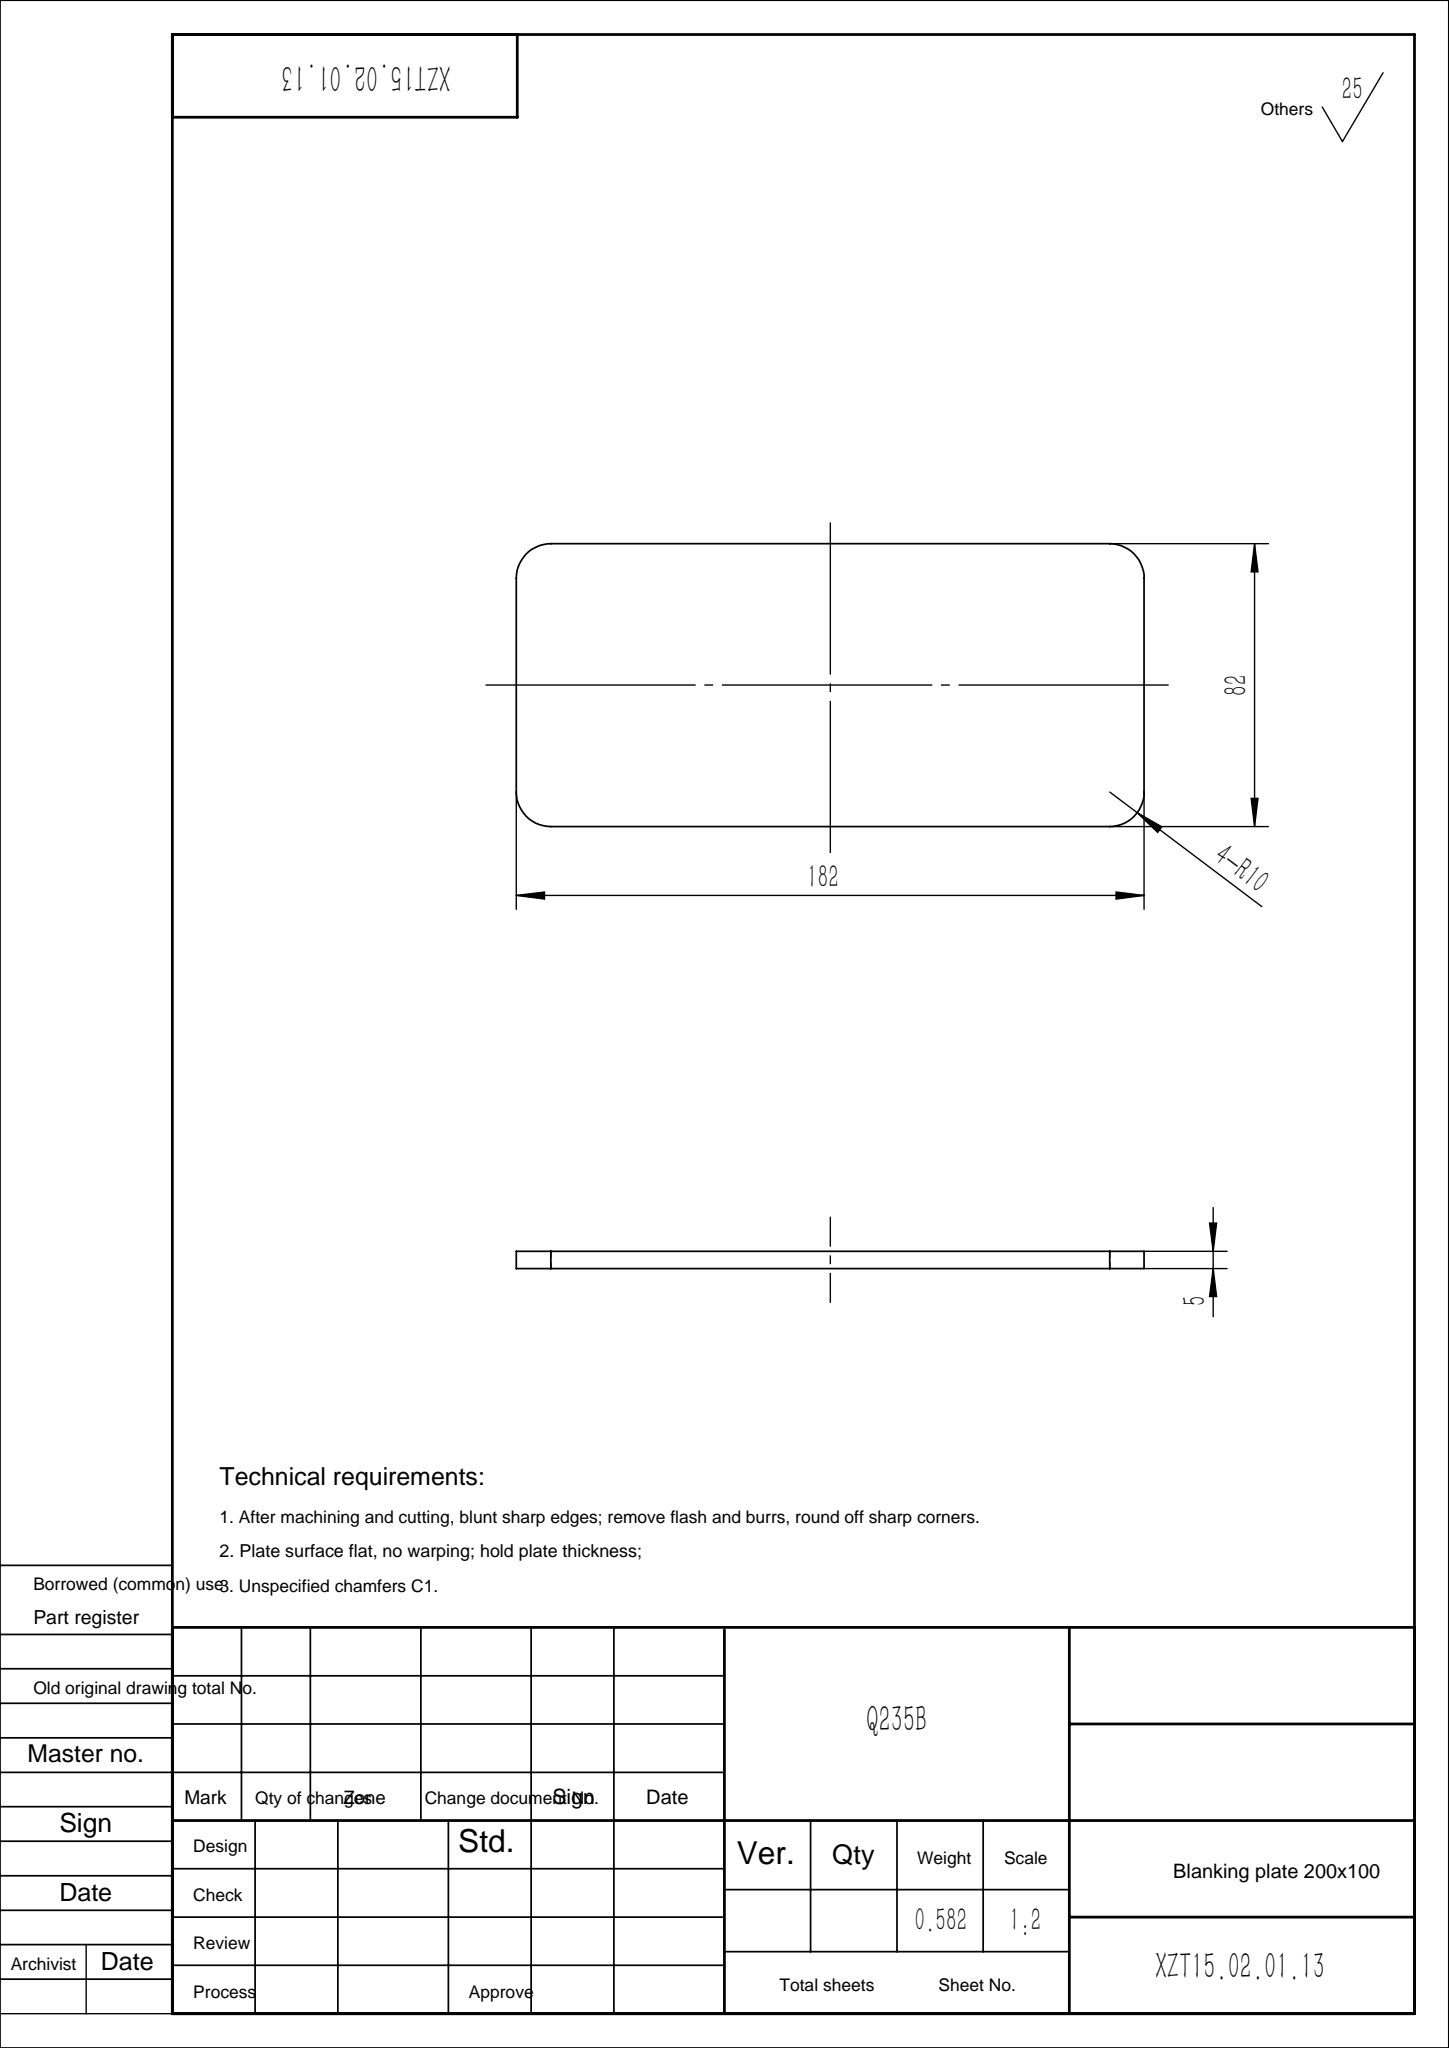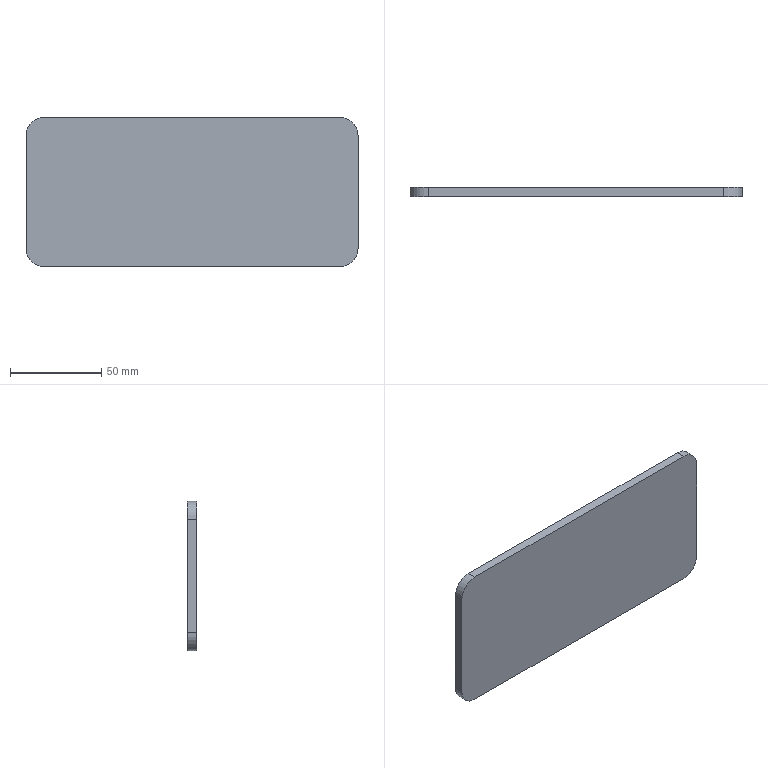Part | SolidWorks | features Chamfer 1, Extrusion 1, Fillet 1, HoleWzd 1 | 1 solid | 10 faces | box 182 x 5 x 82 mm | volume 74191 mm3 | plane 6 | cylinder 4 | commonest cylinder face diameters 20 x4
STEP:
#1=CARTESIAN_POINT('',(-91.,0.,-31.));
#2=VERTEX_POINT('',#1);
#3=CARTESIAN_POINT('',(-91.,0.,31.));
#4=VERTEX_POINT('',#3);
#5=CARTESIAN_POINT('',(-91.,0.,41.));
#6=DIRECTION('',(0.,0.,1.));
#7=VECTOR('',#6,1000.);
#8=LINE('',#5,#7);
#9=EDGE_CURVE('',#2,#4,#8,.T.);
#10=ORIENTED_EDGE('',*,*,#9,.T.);
#11=CARTESIAN_POINT('',(-91.,5.,31.));
#12=VERTEX_POINT('',#11);
#13=CARTESIAN_POINT('',(-91.,5.,31.));
#14=DIRECTION('',(0.,1.,0.));
#15=VECTOR('',#14,1000.);
#16=LINE('',#13,#15);
#17=EDGE_CURVE('',#4,#12,#16,.T.);
#18=ORIENTED_EDGE('',*,*,#17,.T.);
#19=CARTESIAN_POINT('',(-91.,5.,-31.));
#20=VERTEX_POINT('',#19);
#21=CARTESIAN_POINT('',(-91.,5.,41.));
#22=DIRECTION('',(0.,0.,1.));
#23=VECTOR('',#22,1000.);
#24=LINE('',#21,#23);
#25=EDGE_CURVE('',#20,#12,#24,.T.);
#26=ORIENTED_EDGE('',*,*,#25,.F.);
#27=CARTESIAN_POINT('',(-91.,5.,-31.));
#28=DIRECTION('',(0.,-1.,0.));
#29=VECTOR('',#28,1000.);
#30=LINE('',#27,#29);
#31=EDGE_CURVE('',#20,#2,#30,.T.);
#32=ORIENTED_EDGE('',*,*,#31,.T.);
#33=EDGE_LOOP('',(#10,#18,#26,#32));
#34=FACE_OUTER_BOUND('',#33,.T.);
#35=CARTESIAN_POINT('',(-91.,5.,41.));
#36=DIRECTION('',(1.,0.,0.));
#37=DIRECTION('',(0.,0.,-1.));
#38=AXIS2_PLACEMENT_3D('',#35,#36,#37);
#39=PLANE('',#38);
#40=ADVANCED_FACE('',(#34),#39,.F.);
#41=CARTESIAN_POINT('',(-81.,0.,41.));
#42=VERTEX_POINT('',#41);
#43=CARTESIAN_POINT('',(81.,0.,41.));
#44=VERTEX_POINT('',#43);
#45=CARTESIAN_POINT('',(91.,0.,41.));
#46=DIRECTION('',(1.,0.,0.));
#47=VECTOR('',#46,1000.);
#48=LINE('',#45,#47);
#49=EDGE_CURVE('',#42,#44,#48,.T.);
#50=ORIENTED_EDGE('',*,*,#49,.T.);
#51=CARTESIAN_POINT('',(81.,5.,41.));
#52=VERTEX_POINT('',#51);
#53=CARTESIAN_POINT('',(81.,5.,41.));
#54=DIRECTION('',(0.,1.,0.));
#55=VECTOR('',#54,1000.);
#56=LINE('',#53,#55);
#57=EDGE_CURVE('',#44,#52,#56,.T.);
#58=ORIENTED_EDGE('',*,*,#57,.T.);
#59=CARTESIAN_POINT('',(-81.,5.,41.));
#60=VERTEX_POINT('',#59);
#61=CARTESIAN_POINT('',(91.,5.,41.));
#62=DIRECTION('',(1.,0.,0.));
#63=VECTOR('',#62,1000.);
#64=LINE('',#61,#63);
#65=EDGE_CURVE('',#60,#52,#64,.T.);
#66=ORIENTED_EDGE('',*,*,#65,.F.);
#67=CARTESIAN_POINT('',(-81.,5.,41.));
#68=DIRECTION('',(0.,-1.,0.));
#69=VECTOR('',#68,1000.);
#70=LINE('',#67,#69);
#71=EDGE_CURVE('',#60,#42,#70,.T.);
#72=ORIENTED_EDGE('',*,*,#71,.T.);
#73=EDGE_LOOP('',(#50,#58,#66,#72));
#74=FACE_OUTER_BOUND('',#73,.T.);
#75=CARTESIAN_POINT('',(91.,5.,41.));
#76=DIRECTION('',(0.,0.,-1.));
#77=DIRECTION('',(-1.,0.,0.));
#78=AXIS2_PLACEMENT_3D('',#75,#76,#77);
#79=PLANE('',#78);
#80=ADVANCED_FACE('',(#74),#79,.F.);
#81=CARTESIAN_POINT('',(91.,0.,31.));
#82=VERTEX_POINT('',#81);
#83=CARTESIAN_POINT('',(91.,0.,-31.));
#84=VERTEX_POINT('',#83);
#85=CARTESIAN_POINT('',(91.,0.,41.));
#86=DIRECTION('',(0.,0.,-1.));
#87=VECTOR('',#86,1000.);
#88=LINE('',#85,#87);
#89=EDGE_CURVE('',#82,#84,#88,.T.);
#90=ORIENTED_EDGE('',*,*,#89,.T.);
#91=CARTESIAN_POINT('',(91.,5.,-31.));
#92=VERTEX_POINT('',#91);
#93=CARTESIAN_POINT('',(91.,5.,-31.));
#94=DIRECTION('',(0.,1.,0.));
#95=VECTOR('',#94,1000.);
#96=LINE('',#93,#95);
#97=EDGE_CURVE('',#84,#92,#96,.T.);
#98=ORIENTED_EDGE('',*,*,#97,.T.);
#99=CARTESIAN_POINT('',(91.,5.,31.));
#100=VERTEX_POINT('',#99);
#101=CARTESIAN_POINT('',(91.,5.,41.));
#102=DIRECTION('',(0.,0.,-1.));
#103=VECTOR('',#102,1000.);
#104=LINE('',#101,#103);
#105=EDGE_CURVE('',#100,#92,#104,.T.);
#106=ORIENTED_EDGE('',*,*,#105,.F.);
#107=CARTESIAN_POINT('',(91.,5.,31.));
#108=DIRECTION('',(0.,-1.,0.));
#109=VECTOR('',#108,1000.);
#110=LINE('',#107,#109);
#111=EDGE_CURVE('',#100,#82,#110,.T.);
#112=ORIENTED_EDGE('',*,*,#111,.T.);
#113=EDGE_LOOP('',(#90,#98,#106,#112));
#114=FACE_OUTER_BOUND('',#113,.T.);
#115=CARTESIAN_POINT('',(91.,5.,41.));
#116=DIRECTION('',(-1.,0.,0.));
#117=DIRECTION('',(0.,0.,1.));
#118=AXIS2_PLACEMENT_3D('',#115,#116,#117);
#119=PLANE('',#118);
#120=ADVANCED_FACE('',(#114),#119,.F.);
#121=CARTESIAN_POINT('',(81.,5.,-41.));
#122=VERTEX_POINT('',#121);
#123=CARTESIAN_POINT('',(-81.,5.,-41.));
#124=VERTEX_POINT('',#123);
#125=CARTESIAN_POINT('',(91.,5.,-41.));
#126=DIRECTION('',(-1.,0.,0.));
#127=VECTOR('',#126,1000.);
#128=LINE('',#125,#127);
#129=EDGE_CURVE('',#122,#124,#128,.T.);
#130=ORIENTED_EDGE('',*,*,#129,.F.);
#131=CARTESIAN_POINT('',(81.,0.,-41.));
#132=VERTEX_POINT('',#131);
#133=CARTESIAN_POINT('',(81.,5.,-41.));
#134=DIRECTION('',(0.,-1.,0.));
#135=VECTOR('',#134,1000.);
#136=LINE('',#133,#135);
#137=EDGE_CURVE('',#122,#132,#136,.T.);
#138=ORIENTED_EDGE('',*,*,#137,.T.);
#139=CARTESIAN_POINT('',(-81.,0.,-41.));
#140=VERTEX_POINT('',#139);
#141=CARTESIAN_POINT('',(91.,0.,-41.));
#142=DIRECTION('',(-1.,0.,0.));
#143=VECTOR('',#142,1000.);
#144=LINE('',#141,#143);
#145=EDGE_CURVE('',#132,#140,#144,.T.);
#146=ORIENTED_EDGE('',*,*,#145,.T.);
#147=CARTESIAN_POINT('',(-81.,5.,-41.));
#148=DIRECTION('',(0.,1.,0.));
#149=VECTOR('',#148,1000.);
#150=LINE('',#147,#149);
#151=EDGE_CURVE('',#140,#124,#150,.T.);
#152=ORIENTED_EDGE('',*,*,#151,.T.);
#153=EDGE_LOOP('',(#130,#138,#146,#152));
#154=FACE_OUTER_BOUND('',#153,.T.);
#155=CARTESIAN_POINT('',(91.,5.,-41.));
#156=DIRECTION('',(0.,0.,1.));
#157=DIRECTION('',(1.,0.,0.));
#158=AXIS2_PLACEMENT_3D('',#155,#156,#157);
#159=PLANE('',#158);
#160=ADVANCED_FACE('',(#154),#159,.F.);
#161=ORIENTED_EDGE('',*,*,#105,.T.);
#162=CARTESIAN_POINT('',(81.,5.,-31.));
#163=DIRECTION('',(0.,1.,0.));
#164=DIRECTION('',(0.,0.,1.));
#165=AXIS2_PLACEMENT_3D('',#162,#163,#164);
#166=CIRCLE('',#165,10.);
#167=EDGE_CURVE('',#92,#122,#166,.T.);
#168=ORIENTED_EDGE('',*,*,#167,.T.);
#169=ORIENTED_EDGE('',*,*,#129,.T.);
#170=CARTESIAN_POINT('',(-81.,5.,-31.));
#171=DIRECTION('',(0.,1.,0.));
#172=DIRECTION('',(0.,0.,1.));
#173=AXIS2_PLACEMENT_3D('',#170,#171,#172);
#174=CIRCLE('',#173,10.);
#175=EDGE_CURVE('',#124,#20,#174,.T.);
#176=ORIENTED_EDGE('',*,*,#175,.T.);
#177=ORIENTED_EDGE('',*,*,#25,.T.);
#178=CARTESIAN_POINT('',(-81.,5.,31.));
#179=DIRECTION('',(0.,1.,0.));
#180=DIRECTION('',(0.,0.,1.));
#181=AXIS2_PLACEMENT_3D('',#178,#179,#180);
#182=CIRCLE('',#181,10.);
#183=EDGE_CURVE('',#12,#60,#182,.T.);
#184=ORIENTED_EDGE('',*,*,#183,.T.);
#185=ORIENTED_EDGE('',*,*,#65,.T.);
#186=CARTESIAN_POINT('',(81.,5.,31.));
#187=DIRECTION('',(0.,1.,0.));
#188=DIRECTION('',(0.,0.,1.));
#189=AXIS2_PLACEMENT_3D('',#186,#187,#188);
#190=CIRCLE('',#189,10.);
#191=EDGE_CURVE('',#52,#100,#190,.T.);
#192=ORIENTED_EDGE('',*,*,#191,.T.);
#193=EDGE_LOOP('',(#161,#168,#169,#176,#177,#184,#185,#192));
#194=FACE_OUTER_BOUND('',#193,.T.);
#195=CARTESIAN_POINT('',(0.,5.,0.));
#196=DIRECTION('',(0.,1.,0.));
#197=DIRECTION('',(0.,0.,1.));
#198=AXIS2_PLACEMENT_3D('',#195,#196,#197);
#199=PLANE('',#198);
#200=ADVANCED_FACE('',(#194),#199,.T.);
#201=ORIENTED_EDGE('',*,*,#145,.F.);
#202=CARTESIAN_POINT('',(81.,0.,-31.));
#203=DIRECTION('',(0.,-1.,0.));
#204=DIRECTION('',(0.,0.,1.));
#205=AXIS2_PLACEMENT_3D('',#202,#203,#204);
#206=CIRCLE('',#205,10.);
#207=EDGE_CURVE('',#132,#84,#206,.T.);
#208=ORIENTED_EDGE('',*,*,#207,.T.);
#209=ORIENTED_EDGE('',*,*,#89,.F.);
#210=CARTESIAN_POINT('',(81.,0.,31.));
#211=DIRECTION('',(0.,-1.,0.));
#212=DIRECTION('',(0.,0.,1.));
#213=AXIS2_PLACEMENT_3D('',#210,#211,#212);
#214=CIRCLE('',#213,10.);
#215=EDGE_CURVE('',#82,#44,#214,.T.);
#216=ORIENTED_EDGE('',*,*,#215,.T.);
#217=ORIENTED_EDGE('',*,*,#49,.F.);
#218=CARTESIAN_POINT('',(-81.,0.,31.));
#219=DIRECTION('',(0.,-1.,0.));
#220=DIRECTION('',(0.,0.,1.));
#221=AXIS2_PLACEMENT_3D('',#218,#219,#220);
#222=CIRCLE('',#221,10.);
#223=EDGE_CURVE('',#42,#4,#222,.T.);
#224=ORIENTED_EDGE('',*,*,#223,.T.);
#225=ORIENTED_EDGE('',*,*,#9,.F.);
#226=CARTESIAN_POINT('',(-81.,0.,-31.));
#227=DIRECTION('',(0.,-1.,0.));
#228=DIRECTION('',(0.,0.,1.));
#229=AXIS2_PLACEMENT_3D('',#226,#227,#228);
#230=CIRCLE('',#229,10.);
#231=EDGE_CURVE('',#2,#140,#230,.T.);
#232=ORIENTED_EDGE('',*,*,#231,.T.);
#233=EDGE_LOOP('',(#201,#208,#209,#216,#217,#224,#225,#232));
#234=FACE_OUTER_BOUND('',#233,.T.);
#235=CARTESIAN_POINT('',(0.,0.,0.));
#236=DIRECTION('',(0.,1.,0.));
#237=DIRECTION('',(0.,0.,1.));
#238=AXIS2_PLACEMENT_3D('',#235,#236,#237);
#239=PLANE('',#238);
#240=ADVANCED_FACE('',(#234),#239,.F.);
#241=ORIENTED_EDGE('',*,*,#167,.F.);
#242=ORIENTED_EDGE('',*,*,#97,.F.);
#243=ORIENTED_EDGE('',*,*,#207,.F.);
#244=ORIENTED_EDGE('',*,*,#137,.F.);
#245=EDGE_LOOP('',(#241,#242,#243,#244));
#246=FACE_OUTER_BOUND('',#245,.T.);
#247=CARTESIAN_POINT('',(81.,5.,-31.));
#248=DIRECTION('',(0.,-1.,0.));
#249=DIRECTION('',(0.,0.,-1.));
#250=AXIS2_PLACEMENT_3D('',#247,#248,#249);
#251=CYLINDRICAL_SURFACE('',#250,10.);
#252=ADVANCED_FACE('',(#246),#251,.T.);
#253=ORIENTED_EDGE('',*,*,#191,.F.);
#254=ORIENTED_EDGE('',*,*,#57,.F.);
#255=ORIENTED_EDGE('',*,*,#215,.F.);
#256=ORIENTED_EDGE('',*,*,#111,.F.);
#257=EDGE_LOOP('',(#253,#254,#255,#256));
#258=FACE_OUTER_BOUND('',#257,.T.);
#259=CARTESIAN_POINT('',(81.,5.,31.));
#260=DIRECTION('',(0.,-1.,0.));
#261=DIRECTION('',(0.,0.,-1.));
#262=AXIS2_PLACEMENT_3D('',#259,#260,#261);
#263=CYLINDRICAL_SURFACE('',#262,10.);
#264=ADVANCED_FACE('',(#258),#263,.T.);
#265=ORIENTED_EDGE('',*,*,#183,.F.);
#266=ORIENTED_EDGE('',*,*,#17,.F.);
#267=ORIENTED_EDGE('',*,*,#223,.F.);
#268=ORIENTED_EDGE('',*,*,#71,.F.);
#269=EDGE_LOOP('',(#265,#266,#267,#268));
#270=FACE_OUTER_BOUND('',#269,.T.);
#271=CARTESIAN_POINT('',(-81.,5.,31.));
#272=DIRECTION('',(0.,-1.,0.));
#273=DIRECTION('',(0.,0.,-1.));
#274=AXIS2_PLACEMENT_3D('',#271,#272,#273);
#275=CYLINDRICAL_SURFACE('',#274,10.);
#276=ADVANCED_FACE('',(#270),#275,.T.);
#277=ORIENTED_EDGE('',*,*,#175,.F.);
#278=ORIENTED_EDGE('',*,*,#151,.F.);
#279=ORIENTED_EDGE('',*,*,#231,.F.);
#280=ORIENTED_EDGE('',*,*,#31,.F.);
#281=EDGE_LOOP('',(#277,#278,#279,#280));
#282=FACE_OUTER_BOUND('',#281,.T.);
#283=CARTESIAN_POINT('',(-81.,5.,-31.));
#284=DIRECTION('',(0.,-1.,0.));
#285=DIRECTION('',(0.,0.,-1.));
#286=AXIS2_PLACEMENT_3D('',#283,#284,#285);
#287=CYLINDRICAL_SURFACE('',#286,10.);
#288=ADVANCED_FACE('',(#282),#287,.T.);
#289=CLOSED_SHELL('',(#40,#80,#120,#160,#200,#240,#252,#264,#276,#288));
#290=MANIFOLD_SOLID_BREP('',#289);
#291=CARTESIAN_POINT('',(0.,0.,0.));
#292=DIRECTION('',(0.,0.,1.));
#293=DIRECTION('',(1.,0.,0.));
#294=AXIS2_PLACEMENT_3D('',#291,#292,#293);
#295=(LENGTH_UNIT()NAMED_UNIT(*)SI_UNIT(.MILLI.,.METRE.));
#296=UNCERTAINTY_MEASURE_WITH_UNIT(LENGTH_MEASURE(0.00001),#295,'','');
#297=(NAMED_UNIT(*)PLANE_ANGLE_UNIT()SI_UNIT($,.RADIAN.));
#298=(NAMED_UNIT(*)SI_UNIT($,.STERADIAN.)SOLID_ANGLE_UNIT());
#299=(GEOMETRIC_REPRESENTATION_CONTEXT(3)GLOBAL_UNCERTAINTY_ASSIGNED_CONTEXT((#296))GLOBAL_UNIT_ASSIGNED_CONTEXT((#295,#297,#298))REPRESENTATION_CONTEXT('',''));
#300=ADVANCED_BREP_SHAPE_REPRESENTATION('',(#290,#294),#299);